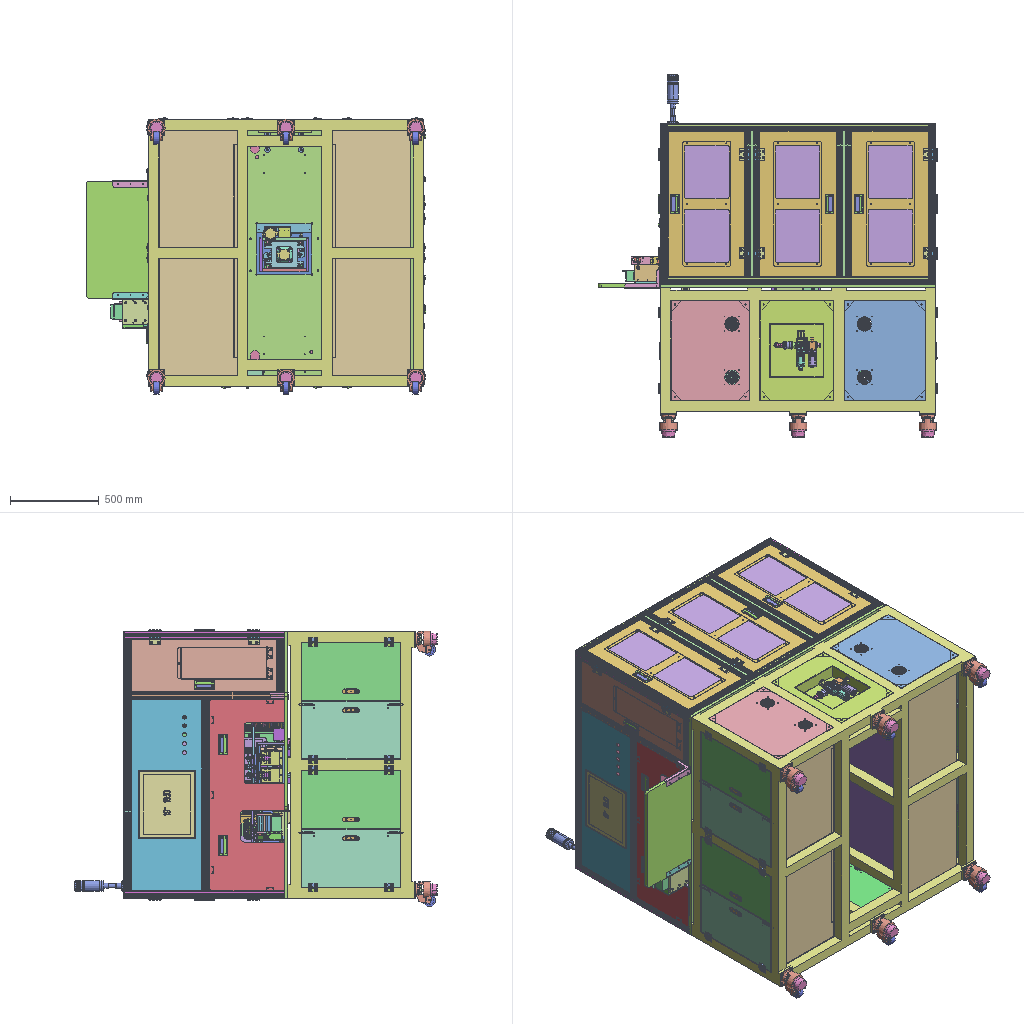Assembly | STEP file | 382 different items | 1685 placed | box 1911 x 2039 x 1557 mm
Parts list (item | name | quantity | parent item | size | volume), first 223 of 382 items:
1 | 01-01 loading base plate | x2 | in 01-00-01 loading module, 01-00-01 Upper料模组-1 | 290 x 20 x 23 mm | 111051 mm3
2 | 01-02 loading sliding plate | x2 | in 01-00-01 loading module, 01-00-01 Upper料模组-1 | 62 x 42 x 235 mm | 266877 mm3
3 | 01-02-01 fibre mounting seat | x2 | in 01-00-01 loading module, 01-00-01 Upper料模组-1 | 16 x 15 x 6 mm | 1218 mm3
4 | 01-03 loading sliding base plate | x2 | in 01-00-01 loading module, 01-00-01 Upper料模组-1 | 290 x 62 x 10 mm | 166343 mm3
5 | 01-04 cylinder pad block | x2 | in 01-00-01 loading module, 01-00-01 Upper料模组-1 | 62 x 40 x 9.5 mm | 22560 mm3
6 | 01-05 small base plate | x2 | in 01-00-01 loading module, 01-00-01 Upper料模组-1 | 290 x 15 x 80 mm | 328016 mm3
7 | 01-06 sliding guide post | x8 | in 01-00-01 loading module, 01-00-01 Upper料模组-1 | 8 x 8 x 70 mm | 3411 mm3
8 | 01-07 loading cylinder pad plate | x2 | in 01-00 loading base die assembly | 22.5 x 30 x 5 mm | 3194 mm3
9 | 01-08 small floating joint | x3 | in 01-00 loading base die assembly | 10 x 10 x 18.1 mm | 1056 mm3
10 | 01-09 floating joint fixing plate | x1 | in 01-00 loading base die assembly | 20 x 12 x 35 mm | 2813 mm3
11 | 01-10 floating joint fixing plate A | x1 | in 01-00 loading base die assembly | 20 x 12 x 35 mm | 2813 mm3
12 | 01-11 guard plate (Default) | x2 | in 01-00-01 loading module, 01-00-01 Upper料模组-1 | 116.5 x 83 x 65 mm | 37563 mm3
13 | 01-12 front baffle | x2 | in 01-00-01 loading module, 01-00-01 Upper料模组-1 | 30 x 30 x 5 mm | 4301 mm3
14 | 01-13 loading guide post | x4 | in 01-00-01 loading module, 01-00-01 Upper料模组-1 | 10 x 10 x 100 mm | 7447 mm3
15 | 01-14 side plate | x2 | in 01-00 loading base die assembly | 149.5 x 180 x 10 mm | 267445 mm3
16 | 01-15 cover plate | x1 | in 01-00 loading base die assembly | 270 x 180 x 6 mm | 290112 mm3
17 | 01-16 side baffle (Default) | x4 | in 01-00-01 loading module, 01-00-01 Upper料模组-1 | 203 x 32.995 x 1.966 mm | 5739 mm3
18 | 02-01 module support plate A | x1 | in 02-00 inspection assembly A | 210 x 80 x 12 mm | 192896 mm3
19 | 02-02 camera fixing side plate | x2 | in 02-00 inspection assembly A | 121.5 x 66 x 10 mm | 61611 mm3
20 | 02-03 buffer pad block | x4 | in 02-00-Y axis assembly, 02-00-Y轴Component-1 | 14 x 7 x 14 mm | 808.175 mm3
21 | 02-04 corrugated tube mounting seat (Default) | x2 | in 02-00 incoming inspection station, 02-00 inspection assembly A | 40 x 70 x 2 mm | 4109 mm3
22 | 02-05 camera fixing plate | x1 | in 02-00 inspection assembly A | 90 x 90 x 10 mm | 76368 mm3
23 | 02-06 product suction plate b | x1 | in 02-00 waste suction mechanism | 98.778 x 46.377 x 10 mm | 12156 mm3
24 | 02-07 product suction plate C | x1 | in 02-00 waste suction mechanism | 98.778 x 46.377 x 10 mm | 11497 mm3
25 | 02-08 gripper limit block | x1 | in 02-00 waste suction mechanism | 32 x 50 x 20 mm | 12367 mm3
26 | 02-09 moving fixing plate | x4 | in 02-00-Y axis assembly, 02-00-Y轴Component-1 | 69.4 x 87 x 10 mm | 57942 mm3
27 | 02-10 corrugated tube mounting plate (Default) | x1 | in 02-00 inspection assembly A | 40 x 52 x 40 mm | 5649 mm3
28 | 02-11 reject box (Default_as machined_) | x1 | in 02-00 inspection assembly A | 148 x 218 x 48 mm | 83489 mm3
29 | 02-12 sensor stop plate (Default) | x2 | in 02-00-Y axis assembly, 02-00-Y轴Component-1 | 15 x 18 x 6.5 mm | 315.442 mm3
30 | 02-13Y轴底Plate | x2 | in 02-00-Y axis assembly, 02-00-Y轴Component-1 | 310 x 87 x 8 mm | 147659 mm3
31 | 02-14 pad block | x4 | in 02-00-Y axis assembly, 02-00-Y轴Component-1 | 8 x 8 x 8 mm | 274.889 mm3
32 | 02-15 tensioning shaft | x2 | in 02-00-Y axis assembly, 02-00-Y轴Component-1 | 9 x 37 x 8 mm | 1080 mm3
33 | 02-16 washer | x2 | in 02-00-Y axis assembly, 02-00-Y轴Component-1 | 8 x 8 x 2 mm | 34.165 mm3
34 | 02-17 timing belt fixing block | x2 | in 02-00-Y axis assembly, 02-00-Y轴Component-1 | 35 x 17 x 11 mm | 5983 mm3
35 | 02-18 press plate | x2 | in 02-00-Y axis assembly, 02-00-Y轴Component-1 | 35 x 17 x 2 mm | 1160 mm3
36 | 02-19 slide table plate | x2 | in 02-00-Y axis assembly, 02-00-Y轴Component-1 | 80 x 78 x 10 mm | 42678 mm3
37 | 02-20 scrap support plate (Default) | x2 | in 02-00 inspection assembly A | 90 x 30 x 30 mm | 10166 mm3
38 | 02-21 vacuum gauge mounting seat (Default) | x1 | in 02-00 incoming inspection station | 70 x 72 x 21.5 mm | 8092 mm3
39 | 03-01 trimming base die | x1 | in 03-00 trimming base die assembly | 180 x 20 x 120 mm | 352918 mm3
40 | 03-02 left cutter pad block | x2 | in 03-00 trimming base die assembly | 14 x 18.7 x 12 mm | 2273 mm3
41 | 03-03 right cutter pad block | x2 | in 03-00 trimming base die assembly | 14 x 18.95 x 12 mm | 2331 mm3
42 | 03-04 cutter pad block press plate | x2 | in 03-00 trimming base die assembly | 30 x 3 x 12 mm | 896.818 mm3
43 | 03-05 cutter fixing plate | x1 | in 03-00 trimming base die assembly | 138.5 x 10 x 77 mm | 77712 mm3
44 | 03-06 right pre-press cutter plate | x2 | in 03-00 trimming upper die assembly | 15 x 25 x 25 mm | 5962 mm3
45 | 03-07 lower cutter | x4 | in 03-00 trimming base die assembly | 4.5 x 3.5 x 37 mm | 428.1 mm3
46 | 03-08 left pre-press cutter plate | x2 | in 03-00 trimming upper die assembly | 15 x 25 x 25 mm | 5712 mm3
47 | 03-09 lift cylinder limit ring | x1 | in 03-00 trimming base die assembly | 12 x 12 x 8 mm | 639.314 mm3
48 | 03-10 cylinder limit post | x3 | in 03-00 trimming upper die assembly | 12 x 12 x 30 mm | 3278 mm3
49 | 03-11 upper blade limit block | x4 | in 03-00 trimming upper die assembly | 30 x 15 x 15 mm | 4822 mm3
50 | 03-12 trimming upper-left blade | x2 | in 03-00 trimming upper die assembly | 7.5 x 9 x 51.3 mm | 2999 mm3
51 | 03-13 trimming upper blade base plate | x1 | in 03-00 trimming upper die assembly | 180 x 120 x 20 mm | 311615 mm3
52 | 03-14 trimming upper-right blade | x2 | in 03-00 trimming upper die assembly | 7 x 9 x 51 mm | 2452 mm3
53 | 03-15 trimming support plate | x2 | in 03-00 trimming base die assembly | 180 x 60 x 12 mm | 114271 mm3
54 | 03-16 trimming support bracket | x1 | in 03-00 trimming base die assembly | 180 x 120 x 10 mm | 134253 mm3
55 | 03-17 trimming upper support bracket | x2 | in 03-00 trimming upper die assembly | 120 x 30 x 12 mm | 41120 mm3
56 | 03-18 guide post A | x4 | in 03-00 trimming base die assembly | 6 x 6 x 22 mm | 567.268 mm3
57 | 03-19 sensor press plate | x10 | in 03-00 trimming base die assembly, 04-00 left bending assembly, 07-00 runout base die, 07-00偏摆度底模-2, 07-00偏摆度底模-3 | 20 x 8 x 3 mm | 387.026 mm3
58 | 03-20 product pre-press block | x2 | in 03-00 trimming upper die assembly | 55 x 20 x 20 mm | 15350 mm3
59 | 03-21 guide screw | x4 | in 03-00 trimming upper die assembly | 8 x 48 x 8 mm | 1019 mm3
60 | 03-22 support plate | x2 | in 03-00 trimming base die assembly | 120 x 30 x 12 mm | 40909 mm3
61 | 03-23 support bracket | x5 | in 03-00 trimming base die assembly, 07-00 runout base die, 07-00偏摆度底模-1, 07-00偏摆度底模-2, 07-00偏摆度底模-3 | 210 x 120 x 12 mm | 293652 mm3
62 | 03-24 side guard plate | x2 | in 03-00 trimming base die assembly | 120 x 60 x 3 mm | 21345 mm3
63 | 03-25 scrap box (Default) | x1 | in 03-00 trimming base die assembly | 153 x 168 x 50 mm | 66699 mm3
64 | 03-26压机底Plate | x9 | in 01-00 loading base die assembly, 02-00 inspection assembly A, 03-00 press, 04-00 pressure-holding assembly, 04-00保压Component-1, 06-00 camera fixing bracket, 07-00 camera fixing bracket, 08-00 unloading station | 250 x 270 x 12 mm | 774847 mm3
65 | 03-27 post B | x4 | in 03-00 press | 25 x 25 x 370 mm | 178727 mm3
66 | 03-28 press moving plate | x1 | in 03-00 press | 250 x 270 x 15 mm | 814940 mm3
67 | 03-29 press fixed plate | x1 | in 03-00 press | 250 x 150 x 12 mm | 428713 mm3
68 | 03-30SC气缸垫块 | x1 | in 03-00 press | 10 x 90 x 53 mm | 35177 mm3
69 | 03-31SC Floating JointFixed座 | x3 | in 03-00 press, 04-00 pressure-holding assembly, 04-00保压Component-1 | 66 x 34 x 17 mm | 26495 mm3
70 | 03-32SC Floating Joint | x1 | in 03-00 press | 26 x 28 x 26 mm | 2635 mm3
71 | 03-33 limit pin | x8 | in 03-00 trimming base die assembly | 0.6 x 0.6 x 2.7 mm | 0.6783 mm3
72 | 03-34 cable tray mounting plate (Default) | x1 | in 03-00 press | 388 x 60 x 11.5 mm | 36165 mm3
73 | 03-35 guide bushing mounting seat | x4 | in 03-00 trimming upper die assembly | 35 x 30 x 10 mm | 5722 mm3
74 | 03-36 iron plate baffle (Default) | x2 | in 03-00 trimming upper die assembly | 29 x 24.5 x 13 mm | 1713 mm3
75 | 03-37 iron plate baffle A (Default) | x2 | in 03-00 trimming upper die assembly | 34 x 24.5 x 15 mm | 2017 mm3
76 | 03-38 cylinder washer | x1 | in 03-00 trimming base die assembly | 16 x 14 x 18 mm | 1876 mm3
77 | 03-39 cutter pad plate | x2 | in 03-00 trimming base die assembly | 31 x 70 x 2 mm | 4295 mm3
78 | 04-01 left bending base die | x1 | in 04-00 left bending assembly | 180 x 20 x 120 mm | 264352 mm3
79 | 04-02 bending swing lever | x4 | in 04-00 bending press head A, 04-00 bending press head B, 04-00 bending press head B-1 | 33.617 x 33.617 x 84.85 mm | 10597 mm3
80 | 04-02-01 left bending mounting plate | x2 | in 04-00 bending press head B, 04-00 bending press head B-1 | 50 x 70 x 15 mm | 38195 mm3
81 | 04-02-02 small base plate | x4 | in 04-00 bending press head B, 04-00 bending press head B-1, 05-00 bending assembly B, 05-00 bending assembly B-1 | 50 x 73.8 x 10 mm | 27452 mm3
82 | 04-02-03 left bending cylinder mounting plate | x4 | in 04-00 bending press head B, 04-00 bending press head B-1, 05-00 bending assembly B, 05-00 bending assembly B-1 | 50 x 70 x 10 mm | 29834 mm3
83 | 04-02-04 small base plate C | x4 | in 04-00 bending press head B, 04-00 bending press head B-1, 05-00 bending assembly B, 05-00 bending assembly B-1 | 70 x 73.8 x 10 mm | 48282 mm3
84 | 04-02-05 adjustment platform base plate | x1 | in 04-00 left bending assembly | 157 x 60 x 10 mm | 92232 mm3
85 | 04-02-06 adjustment base plate | x4 | in 04-00 bending press head B, 04-00 bending press head B-1, 05-00 bending assembly B, 05-00 bending assembly B-1 | 60 x 70 x 10 mm | 39504 mm3
86 | 04-03 bending press head | x4 | in 04-00 bending press head A, 04-00 bending press head B, 04-00 bending press head B-1 | 3.8 x 5.341 x 9.237 mm | 81.885 mm3
87 | 04-04 equal-height profile A | x4 | in 04-00 pressure-holding assembly, 04-00保压Component-1 | 60 x 30 x 315 mm | 207544 mm3
88 | 04-05 bending support plate | x4 | in 04-00 left bending assembly, 05-00 right bending assembly A | 90 x 100 x 12 mm | 106188 mm3
89 | 04-07 bearing retaining ring | x9 | in 04-00 bending press head A, 04-00 bending press head B, 04-00 bending press head B-1, 05-00 bending assembly B, 05-00 bending assembly B-1, 06-00-A rotary fixture, 06-00-A Revolve载具-1, Right bending assembly, Right折弯Component-1 | 8 x 22 x 22 mm | 1770 mm3
90 | 04-08 rotary limit block | x14 | in 04-00 bending press head A, 04-00 bending press head B, 04-00 bending press head B-1, 05-00 bending assembly B, 05-00 bending assembly B-1, Right bending assembly, Right折弯Component-1 | 25 x 10 x 8 mm | 1473 mm3
91 | 04-09 rotary shaft | x3 | in 04-00 bending press head A, Right bending assembly, Right折弯Component-1 | 12 x 12 x 40.9 mm | 2751 mm3
92 | 04-10 bearing mounting seat | x3 | in 04-00 bending press head A, Right bending assembly, Right折弯Component-1 | 50 x 50 x 15 mm | 27889 mm3
93 | 04-11 support stop post | x3 | in 04-00-1 limit post, 04-00-1限位Pillar-1, 04-00-1限位Pillar-2 | 40 x 25 x 15 mm | 11747 mm3
94 | 04-12 support plate | x1 | in 04-00 bending press head A | 50 x 12 x 80 mm | 39354 mm3
95 | 04-13 support plate A | x4 | in 04-00 left bending assembly, 05-00 right bending assembly A | 70 x 60 x 10 mm | 35423 mm3
96 | 04-14 pre-press block | x2 | in 04-00 bending pre-press assembly, 04-00折弯预压Component-1 | 62.5 x 40 x 20 mm | 33897 mm3
97 | 04-14-a pre-press block | x2 | in 04-00 bending pre-press assembly, 04-00折弯预压Component-1 | 62.5 x 40 x 18.7 mm | 34599 mm3
98 | 04-15 guide screw | x14 | in 04-00 bending pre-press assembly, 04-00折弯预压Component-1, 05-00 right bending pre-press assembly, 05-00 Right折弯预压Component-1 | 8 x 38 x 8 mm | 822.389 mm3
99 | 04-16 support bracket | x2 | in 04-00 left bending assembly, 05-00 right bending assembly A | 210 x 185 x 12 mm | 371690 mm3
100 | 04-17 pre-press fixing plate | x2 | in 04-00 pressure-holding assembly, 04-00保压Component-1 | 146.4 x 168 x 10 mm | 235820 mm3
101 | 04-18 small floating joint | x2 | in 04-00 pressure-holding assembly, 04-00保压Component-1 | 26 x 28 x 26 mm | 4043 mm3
102 | 04-19 cylinder connection plate | x2 | in 04-00 pressure-holding assembly, 04-00保压Component-1 | 38 x 64 x 4 mm | 7859 mm3
103 | 04-20 equal-height profile | x4 | in 02-00 inspection assembly A, 07-00 camera fixing bracket | 60 x 30 x 295 mm | 194282 mm3
104 | 04-21 cylinder support bracket | x2 | in 04-00 pressure-holding assembly, 04-00保压Component-1 | 210 x 60 x 12 mm | 122855 mm3
105 | 04-22 guide post | x8 | in 04-00 pressure-holding assembly, 04-00保压Component-1 | 8 x 180 x 8 mm | 8953 mm3
106 | 04-23 belt tensioning plate | x3 | in 04-00 bending press head A, Right bending assembly, Right折弯Component-1 | 30 x 25 x 10 mm | 6603 mm3
107 | 04-24 guide post fixing plate (Default) | x2 | in 04-00 pressure-holding assembly, 04-00保压Component-1 | 150 x 66 x 20 mm | 39207 mm3
108 | 04-25 guide post mounting seat | x1 | in 05-00 right bending mechanism | 21 x 32 x 24 mm | 5053 mm3
109 | 05-01 bending press head | x4 | in 05-00 bending assembly B, 05-00 bending assembly B-1, Right bending assembly, Right折弯Component-1 | 3.8 x 6.694 x 8.962 mm | 82.141 mm3
110 | 05-02 bending swing lever 1 | x6 | in 05-00 bending assembly B, 05-00 bending assembly B-1, Right bending assembly, Right折弯Component-1 | 38.738 x 38.738 x 90.85 mm | 12920 mm3
111 | 05-02-01 rotary fixing plate | x2 | in 05-00 bending assembly B, 05-00 bending assembly B-1 | 60 x 69.2 x 15 mm | 42782 mm3
112 | 05-02-02 adjustment platform base plate | x1 | in 05-00 right bending assembly A | 157 x 60 x 9.5 mm | 87518 mm3
113 | 05-03 left bending base die | x1 | in 05-00 right bending assembly A | 180 x 20 x 120 mm | 280278 mm3
114 | 05-04 bending roller | x22 | in 05-00 bending assembly B, 05-00 bending assembly B-1, Right bending assembly, Right折弯Component-1 | 3.1 x 3.1 x 0.8 mm | 5.41 mm3
115 | 05-05 support plate | x2 | in Right bending assembly, Right折弯Component-1 | 50 x 10.7 x 80 mm | 35177 mm3
116 | 05-06 rotary fixing plate | x2 | in Right bending assembly, Right折弯Component-1 | 60 x 130 x 15 mm | 81399 mm3
117 | 05-07 pre-press block | x2 | in 05-00 right bending pre-press assembly, 05-00 Right折弯预压Component-1 | 60 x 40 x 20 mm | 26248 mm3
118 | 05-07-a pre-press block | x2 | in 05-00 right bending pre-press assembly, 05-00 Right折弯预压Component-1 | 60 x 40 x 18.7 mm | 25800 mm3
119 | 06-01 module pad plate | x1 | in 06-00 camera fixing bracket | 250 x 100 x 15 mm | 368528 mm3
120 | 06-01-02 rotary shaft | x4 | in 06-00-A rotary fixture, 06-00-A Revolve载具-1 | 29 x 20 x 109 mm | 14786 mm3
121 | 06-01-03 rotary base plate | x1 | in 06-00-B rotary fixture assembly | 179 x 106 x 20 mm | 319084 mm3
122 | 06-01-04 rotary shaft sleeve | x2 | in 06-00-A rotary fixture, 06-00-A Revolve载具-1 | 41 x 42 x 72 mm | 36513 mm3
123 | 06-01-05 light source mounting plate A (Default) | x2 | in 06-00-C light source assembly, 06-00-C光源Component-1 | 52 x 41 x 40 mm | 5228 mm3
124 | 06-01-06 support bracket | x1 | in 06-00-B rotary fixture assembly | 210 x 180 x 12 mm | 404728 mm3
125 | 06-01-07 support plate | x2 | in 06-00-B rotary fixture assembly | 120 x 69 x 12 mm | 97250 mm3
126 | 06-01-08 motor pad block | x1 | in 06-00-B rotary fixture assembly | 80 x 25 x 40 mm | 31958 mm3
127 | 06-01-09 light source inclined plate (Default) | x2 | in 06-00-D light source assembly, 06-00-D光源Component-1 | 52 x 32.366 x 13.74 mm | 2941 mm3
128 | 06-01-10 light source inclined plate A (Default) | x2 | in 06-00-D light source assembly, 06-00-D光源Component-1 | 52 x 14.5 x 27.062 mm | 2282 mm3
129 | 06-01-11 fibre mounting seat | x4 | in 06-00-E light source assembly, 06-00-E光源Component-1, 06-00-F fibre fixing seat, 06-00-F光纤Fixed座-1 | 5 x 30 x 5 mm | 550.393 mm3
130 | 06-01-12 laser rotary plate | x2 | in 06-00-F fibre fixing seat, 06-00-F光纤Fixed座-1 | 10 x 21 x 3 mm | 392.466 mm3
131 | 06-01-13 laser rotary plate A | x6 | in 06-00-E light source assembly, 06-00-E光源Component-1, 06-00-F fibre fixing seat, 06-00-F光纤Fixed座-1 | 8 x 8 x 20 mm | 871.542 mm3
132 | 06-01-14 photoelectric sensor plate (Default) | x1 | in 06-00-B rotary fixture assembly | 15 x 15 x 19 mm | 381.957 mm3
133 | 06-01-15 fibre mounting post | x2 | in 06-00-E light source assembly, 06-00-E光源Component-1 | 5 x 60 x 5 mm | 1139 mm3
134 | 06-01-16 light source mounting plate | x2 | in 06-00-E light source assembly, 06-00-E光源Component-1 | 8 x 8 x 49 mm | 1247 mm3
135 | 06-01-17 laser rotary plate B | x2 | in 06-00-E light source assembly, 06-00-E光源Component-1 | 8 x 8 x 28 mm | 1250 mm3
136 | 06-02-01 rotary fixture | x2 | in 06-00-A rotary fixture, 06-00-A Revolve载具-1 | 60 x 30 x 19 mm | 18912 mm3
137 | 06-02-02 light-blocking plate | x3 | in 06-00-A rotary fixture, 06-00-A Revolve载具-1 | 13.3 x 2 x 16.5 mm | 389.932 mm3
138 | 06-02KK60模组连接块 | x2 | in 02-00 inspection assembly A, 06-00 camera fixing bracket | 73 x 70 x 51 mm | 125867 mm3
139 | 06-03 sensor plate | x3 | in 02-00 inspection assembly A, 06-00 camera fixing bracket | 20 x 26 x 1.5 mm | 394.716 mm3
140 | 06-04 sensor mounting strip | x2 | in 02-00 inspection assembly A, 06-00 camera fixing bracket | 15 x 6 x 150 mm | 6689 mm3
141 | 06-05KK60伺服连接Plate(KK60 Upper银伺服连接Plate) | x2 | in 02-00 inspection assembly A, KK60-150A1-F0 | 49.4 x 10 x 40 mm | 11250 mm3
142 | 06-08 light source mounting plate A (Default) | x2 | in 07-00 runout inspection | 52 x 32 x 48 mm | 4676 mm3
143 | 06-09KK60模组连接块 | x1 | in 06-00 camera fixing bracket | 73 x 70 x 12 mm | 52602 mm3
144 | 06-1040 module connection block | x1 | in 06-00 camera fixing bracket | 60 x 70 x 22 mm | 52388 mm3
145 | 06-11 motor flange | x1 | in KK40-100A1-F0 | 40 x 12 x 40 mm | 12158 mm3
146 | 07-01 runout inspection base die | x3 | in 07-00 runout base die, 07-00偏摆度底模-2, 07-00偏摆度底模-3 | 180 x 20 x 120 mm | 238820 mm3
147 | 07-02 support plate | x6 | in 07-00 runout base die, 07-00偏摆度底模-2, 07-00偏摆度底模-3 | 120 x 100 x 12 mm | 141828 mm3
148 | 07-03 camera fixing plate | x5 | in Camera assembly, 相机Assembly-1, 相机Assembly-2, 相机Assembly-3, 相机Assembly-4 | 64 x 90 x 12 mm | 52965 mm3
149 | 07-04 camera mounting plate | x2 | in 06-00 camera fixing bracket, 07-00 camera fixing bracket | 195 x 90 x 10 mm | 166722 mm3
150 | 07-05 triangular support bracket | x2 | in 07-00 camera fixing bracket | 136.5 x 121.3 x 15 mm | 109879 mm3
151 | 07-06 light source bracket (Default) | x5 | in Camera assembly, 相机Assembly-1, 相机Assembly-2, 相机Assembly-3, 相机Assembly-4 | 74 x 71.5 x 170 mm | 24970 mm3
152 | 07-07 light-blocking plate | x10 | in 06-00-A rotary fixture, 06-00-A Revolve载具-1, 07-00 runout base die, 07-00偏摆度底模-1, 07-00偏摆度底模-2, 07-00偏摆度底模-3 | 13.3 x 9.7 x 18.5 mm | 1003 mm3
153 | 07-08LED安装Plate(Default) | x4 | in 07-00 runout inspection | 49 x 11.5 x 15 mm | 1034 mm3
154 | 07-10 reflector plate (Default) | x4 | in 07-00 runout base die, 07-00偏摆度底模-1, 07-00偏摆度底模-2, 07-00偏摆度底模-3 | 13.3 x 14.933 x 10.46 mm | 447.05 mm3
155 | 07-11 locating pin | x24 | in 07-00 runout base die, 07-00偏摆度底模-1, 07-00偏摆度底模-2, 07-00偏摆度底模-3 | 3 x 11 x 3 mm | 70.424 mm3
156 | 08-01 conveyor left baffle | x1 | in 08-01 conveyor assembly | 450 x 136 x 10 mm | 510028 mm3
157 | 08-02 conveyor right baffle | x1 | in 08-01 conveyor assembly | 450 x 136 x 10 mm | 487378 mm3
158 | 08-03 bearing mounting seat | x8 | in 08-02 bearing assembly, 08-02轴承Component-1, 08-02轴承Component-2, 08-02轴承Component-3, 08-02轴承Component-4, 08-02轴承Component-5, 08-02轴承Component-6, 08-02轴承Component-7 | 35 x 35 x 20 mm | 9591 mm3
159 | 08-04 driving shaft | x2 | in 08-01 conveyor assembly | 22 x 22 x 142 mm | 37102 mm3
160 | 08-05 driven shaft | x3 | in 08-01 conveyor assembly | 22 x 22 x 130 mm | 36200 mm3
161 | 08-06 conveyor base plate | x1 | in 08-01 conveyor assembly | 240 x 140 x 15 mm | 481130 mm3
162 | 08-07 limit post | x2 | in 08-01 conveyor assembly | 20 x 20 x 90 mm | 26377 mm3
163 | 08-08 limit block | x6 | in 08-01 conveyor assembly, 08-03 idler assembly, 08-03惰轮Component-1 | 10 x 35 x 10 mm | 2760 mm3
164 | 08-09 idler mounting plate | x2 | in 08-03 idler assembly, 08-03惰轮Component-1 | 60 x 30 x 10 mm | 13911 mm3
165 | 08-10 stop block | x2 | in 08-01 conveyor assembly | 110 x 10 x 10 mm | 9545 mm3
166 | 08-11 shield plate (Default) | x1 | in 08-01 conveyor assembly | 113 x 54.315 x 38.465 mm | 11912 mm3
167 | 08-12 suction plate | x1 | in 08-04 suction cup assembly | 122 x 50 x 10 mm | 31147 mm3
168 | 08-13 rotary support seat | x1 | in 08-04 suction cup assembly | 25 x 22 x 25 mm | 6276 mm3
169 | 08-14 equal-height profile | x1 | in 08-00 unloading station | 60 x 30 x 340 mm | 224122 mm3
170 | 08-18 guard plate (Default) | x1 | in 08-01 conveyor assembly | 402.823 x 48.5 x 131.437 mm | 95492 mm3
171 | 08-19 rotary cylinder mounting plate | x1 | in 08-00 unloading station | 60 x 8 x 70 mm | 24290 mm3
172 | 08-20 rotary support seat | x1 | in 08-04 suction cup assembly | 30 x 30 x 25 mm | 6052 mm3
173 | 08-21 left conveyor adapter plate | x2 | in 08-01 conveyor assembly | 130 x 45 x 10 mm | 48353 mm3
174 | 08-22 side baffle fixing plate | x1 | in 08-01 conveyor assembly | 100 x 50 x 8 mm | 37879 mm3
175 | 08-23 side baffle fixing plate A | x1 | in 08-01 conveyor assembly | 100 x 50 x 8 mm | 37879 mm3
176 | 08-24 recheck collection box (Default_as machined_) | x1 | in 08-01 conveyor assembly | 98 x 163.048 x 60 mm | 52980 mm3
177 | 09-01 table plate | x1 | - | 1550 x 20 x 1500 mm | 43532638 mm3
178 | 09-02 aluminium profile 4040-1470 | x4 | in Upper frame | 40 x 40 x 1470 mm | 1034180 mm3
179 | 09-03 aluminium profile 4040-900 | x4 | in Upper frame | 40 x 40 x 900 mm | 636225 mm3
180 | 09-04 aluminium profile 4040-1420 | x3 | in Upper frame | 40 x 40 x 1420 mm | 998834 mm3
181 | 09-05 aluminium profile 4040-860 | x1 | in Upper frame | 40 x 40 x 860 mm | 605454 mm3
182 | 09-06 aluminium profile 4040-500 | x1 | in Upper frame | 40 x 40 x 300 mm | 207088 mm3
183 | 09-07 upper cover (Default) | x2 | in Upper frame | 775 x 1.5 x 1500 mm | 1741776 mm3
184 | 09-08 panel (Default) | x1 | in Upper frame | 1078 x 398 x 48 mm | 808105 mm3
185 | 09-09 aluminium profile 4080-1420 | x1 | in Upper frame | 40 x 80 x 1420 mm | 1707613 mm3
186 | 09-10 aluminium profile 4040-1080 | x1 | in Upper frame | 40 x 40 x 1080 mm | 758483 mm3
187 | 09-11 upper door B (Default) | x1 | in 09-03 left upper small door | 298 x 818 x 15 mm | 444679 mm3
188 | 09-12 upper door A (Default) | x8 | in 09-02 upper small door, 09-02 Upper小Door-1, 09-02 Upper小Door-2, 09-02 Upper小Door-3, 09-02 Upper小Door-4, 09-02 Upper小Door-5, 09-02 Upper小Door-6, 09-02 Upper小Door-7 | 434 x 818 x 15 mm | 398163 mm3
189 | 09-13 light-transmitting plate | x9 | in 09-02 upper small door, 09-02 Upper小Door-1, 09-02 Upper小Door-2, 09-02 Upper小Door-3, 09-02 Upper小Door-4, 09-02 Upper小Door-5, 09-02 Upper小Door-6, 09-02 Upper小Door-7, 09-04 right upper small door | 270 x 700 x 3 mm | 566234 mm3
190 | 09-14 upper door C (Default) | x1 | in 09-04 right upper small door | 386 x 818 x 15 mm | 335563 mm3
191 | 09-15 aluminium profile 4080-820 | x6 | in Upper frame | 40 x 80 x 820 mm | 984029 mm3
192 | 09-16 lower frame | x1 | in Lower frame | 1550 x 710 x 1500 mm | 100220084 mm3
193 | 09-17 closing plate A (Default) | x1 | in Lower frame | 683 x 558 x 1.5 mm | 563276 mm3
194 | 09-18 closing plate B | x1 | in Lower frame | 683 x 558 x 121.5 mm | 815464 mm3
195 | 09-19 front door panel A (Default) | x4 | in Front left side door panel, 前Left侧DoorPlate-1, 前Left侧DoorPlate-2, 前Left侧DoorPlate-3 | - | -
196 | 09-20 front door panel B (Default) | x4 | in Front right door assembly, 前RightDoorComponent-1, 前RightDoorComponent-2, 前RightDoorComponent-3 | 328 x 558 x 15 mm | 335829 mm3
197 | 09-21 counterweight plate | x4 | in Lower frame | 658 x 438 x 3 mm | 864612 mm3
198 | 09-22 electrical control board | x2 | in Lower frame | 1200 x 540 x 20 mm | 1414884 mm3
199 | 09-23 keyboard bracket (Default) | x1 | in 09-03 left upper small door | 498.5 x 36.5 x 180 mm | 211119 mm3
200 | 09-24 keyboard knob | x1 | in 09-03 left upper small door | 14 x 8 x 10 mm | 897.125 mm3
201 | 09-25 profile fixing bracket | x9 | in Upper frame | 40 x 40 x 45 mm | 29511 mm3
202 | 09-26 closing plate c (Default) | x1 | in Lower frame | 438 x 558 x 1.5 mm | 358211 mm3
203 | 09-27 closing plate D (Default) | x1 | in Lower frame | 453 x 558 x 1.5 mm | 370766 mm3
204 | 09-28 closing plate E (Default) | x1 | in Lower frame | 413 x 558 x 75 mm | 472470 mm3
205 | 09-29 front panel A | x1 | in 09-05 front closing plate A | 1078 x 418 x 5 mm | 1609737 mm3
206 | 09-30 joint adapter plate (Default) | x1 | in Joint assembly | 35 x 2 x 15 mm | 813.303 mm3
207 | 09-31 micro switch seat (Default) | x19 | in Door limit switch assembly, Door限位开关Component-1, Door限位开关Component-10, Door限位开关Component-11, Door限位开关Component-12, Door限位开关Component-13, Door限位开关Component-14, Door限位开关Component-15, Door限位开关Component-16, Door限位开关Component-17, Door限位开关Component-18, Door限位开关Component-2, Door限位开关Component-3, Door限位开关Component-4, Door限位开关Component-5, Door限位开关Component-6, Door限位开关Component-7, Door限位开关Component-8, Door限位开关Component-9 | 25 x 47 x 40 mm | 5190 mm3
208 | 09-34 front table plate | x1 | in Upper frame | 660 x 350 x 20 mm | 4613133 mm3
209 | 09-35 right support plate (Default) | x1 | in Upper frame | 37 x 102 x 200 mm | 31565 mm3
210 | 09-36 left support plate (Default) | x1 | in Upper frame | 200 x 50 x 39 mm | 30286 mm3
211 | 10-01 turntable | x1 | in 10-00 lift and rotate structure | 650 x 8 x 650 mm | 2623771 mm3
212 | 10-02 servo motor mounting seat | x1 | in Rotary shaft assembly | 220 x 197 x 150 mm | 1555452 mm3
213 | 10-03 rotary bearing seat | x1 | in Rotary shaft assembly | 150 x 86 x 150 mm | 549406 mm3
214 | 10-04 bearing seat cover plate upper | x1 | in Rotary shaft assembly | 110 x 37 x 114 mm | 193708 mm3
215 | 10-05 rotary shaft | x1 | in Rotary shaft assembly | 150 x 227 x 150 mm | 734165 mm3
216 | 10-06 shaft shoulder | x1 | in Rotary shaft assembly | 60 x 60 x 11.5 mm | 9808 mm3
217 | 10-07 top ring | x1 | in Rotary shaft assembly | 70 x 14 x 70 mm | 21857 mm3
218 | 10-08 bearing seat cover plate lower | x1 | in Rotary shaft assembly | 114 x 10 x 114 mm | 37218 mm3
219 | 10-09 sensor plate | x8 | in Rotary shaft assembly | 60 x 2 x 95 mm | 4861 mm3
220 | 10-10 sensor fixing block | x1 | in Rotary shaft assembly | 45 x 36 x 20 mm | 7069 mm3
221 | 10-11 lift fixing plate | x2 | in Lifting mechanism | 190 x 280 x 15 mm | 448559 mm3
222 | 10-12 lift fixing plate A | x1 | in Lifting mechanism | 250 x 280 x 15 mm | 827776 mm3
223 | 10-13 lift fixing plate B | x1 | in Lifting mechanism | 250 x 280 x 15 mm | 1044782 mm3